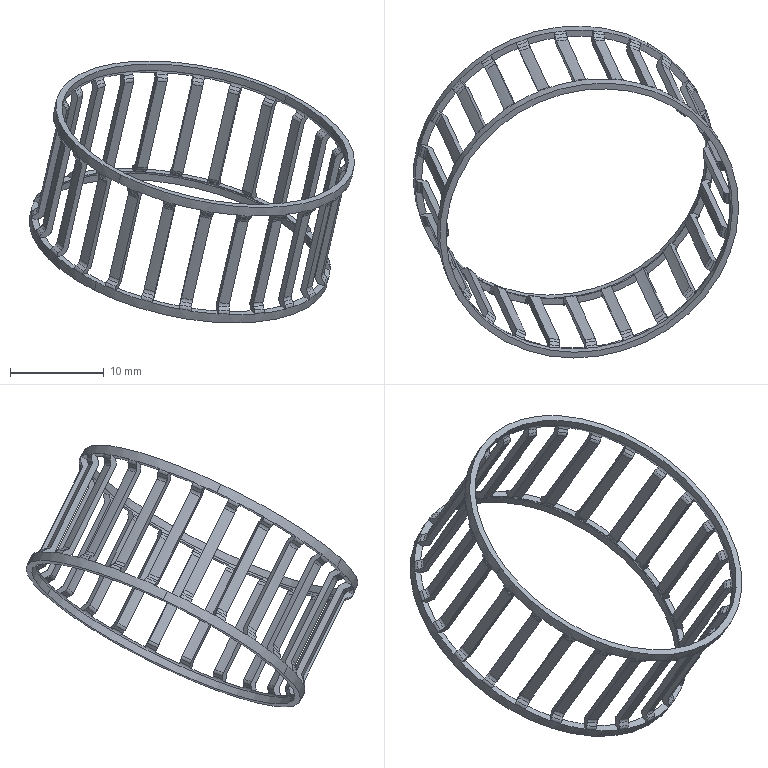Part | SolidWorks | features BaseBody 1 | 1 solid | 404 faces | box 34.658 x 35.361 x 27.908 mm | volume 375.706 mm3 | torus 150 | plane 98 | cone 96 | cylinder 60 | commonest cylinder face diameters 30 x24 31.35 x24 31.15 x6 32.5 x6